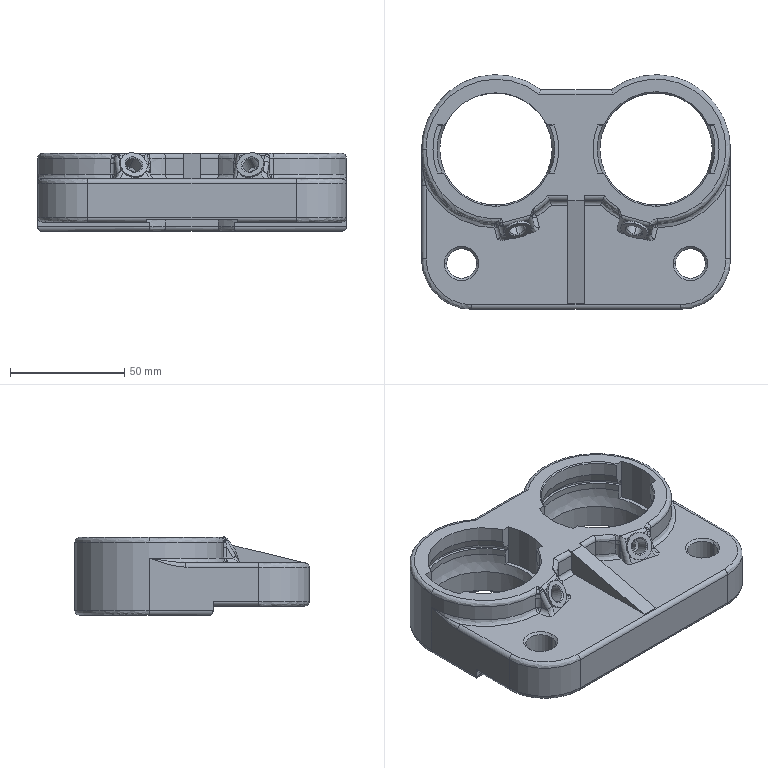Part | SolidWorks | features BaseBody 1 | 1 solid | 222 faces | box 135 x 102.5 x 34.325 mm | volume 207829 mm3 | cylinder 86 | plane 56 | spline 53 | cone 27 | commonest cylinder face diameters 4 x37 49.143 x8 65 x7 54 x6 55 x6 5 x4